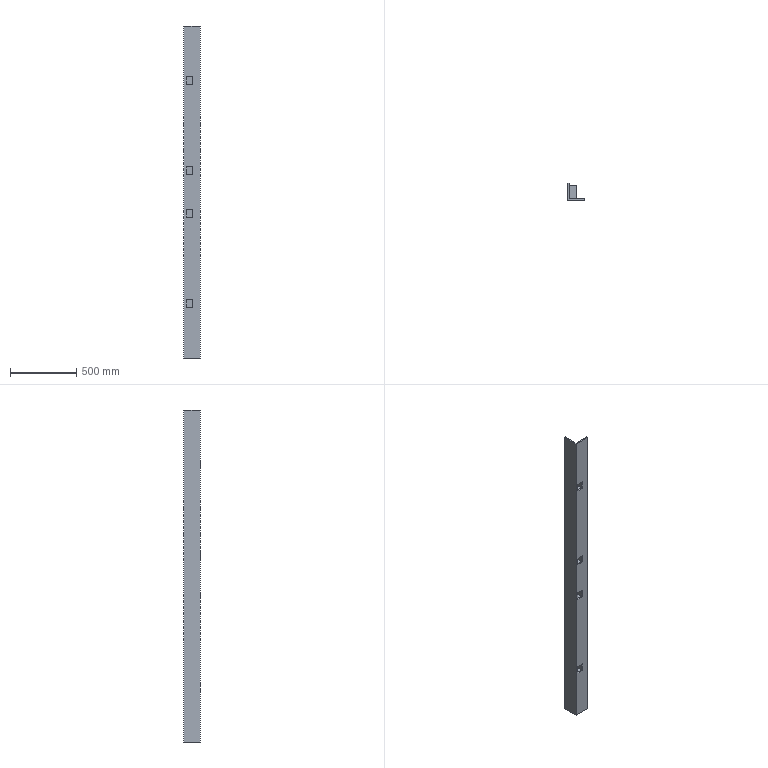Part | SolidWorks | features ICE 2, BossThin 1, Extrusion 1, LPattern 1, MirrorSolid 1 | 9 solids | 88 faces | box 125 x 125 x 2500 mm | volume 6154176 mm3 | plane 88